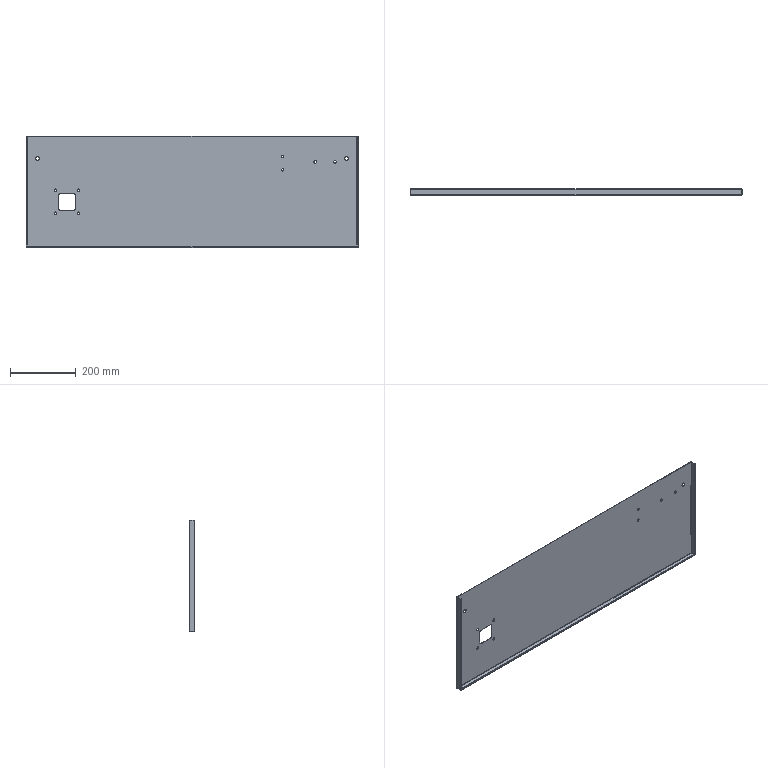Part | SolidWorks | features BaseBody 1 | 1 solid | 74 faces | box 1010 x 18 x 340 mm | volume 447542 mm3 | cylinder 36 | plane 30 | spline 8 | commonest cylinder face diameters 8.5 x12 1.473 x6 3.873 x6 7 x4 10 x4 11 x4